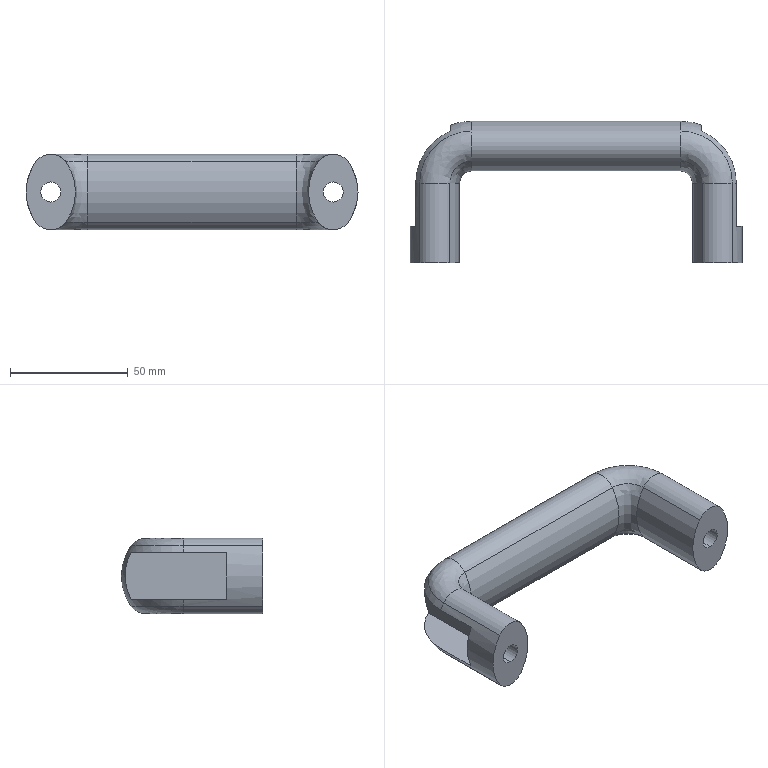Part | SolidWorks | features BaseBody 1 | 1 solid | 43 faces | box 141 x 60 x 32 mm | volume 81760 mm3 | cylinder 23 | plane 12 | spline 8 | commonest cylinder face diameters 16 x9 44.044 x6 8.5 x4 13.5 x4
STEP:
#1=CARTESIAN_POINT('',(-44.25,43.137,-12.848));
#2=VERTEX_POINT('',#1);
#3=CARTESIAN_POINT('',(-44.25,49.5,-16.));
#4=VERTEX_POINT('',#3);
#5=CARTESIAN_POINT('',(-44.25,49.5,-8.));
#6=DIRECTION('',(1.,0.,0.));
#7=DIRECTION('',(0.,0.,-1.));
#8=AXIS2_PLACEMENT_3D('',#5,#6,#7);
#9=CIRCLE('',#8,8.);
#10=EDGE_CURVE('',#2,#4,#9,.T.);
#11=ORIENTED_EDGE('',*,*,#10,.T.);
#12=CARTESIAN_POINT('',(44.25,49.5,-16.));
#13=VERTEX_POINT('',#12);
#14=CARTESIAN_POINT('',(44.25,49.5,-16.));
#15=DIRECTION('',(1.,0.,0.));
#16=VECTOR('',#15,1000.);
#17=LINE('',#14,#16);
#18=EDGE_CURVE('',#4,#13,#17,.T.);
#19=ORIENTED_EDGE('',*,*,#18,.T.);
#20=CARTESIAN_POINT('',(44.25,43.137,-12.848));
#21=VERTEX_POINT('',#20);
#22=CARTESIAN_POINT('',(44.25,49.5,-8.));
#23=DIRECTION('',(-1.,0.,0.));
#24=DIRECTION('',(0.,0.,-1.));
#25=AXIS2_PLACEMENT_3D('',#22,#23,#24);
#26=CIRCLE('',#25,8.);
#27=EDGE_CURVE('',#13,#21,#26,.T.);
#28=ORIENTED_EDGE('',*,*,#27,.T.);
#29=CARTESIAN_POINT('',(44.25,43.137,-12.848));
#30=DIRECTION('',(1.,0.,0.));
#31=VECTOR('',#30,1000.);
#32=LINE('',#29,#31);
#33=EDGE_CURVE('',#2,#21,#32,.T.);
#34=ORIENTED_EDGE('',*,*,#33,.F.);
#35=EDGE_LOOP('',(#11,#19,#28,#34));
#36=FACE_OUTER_BOUND('',#35,.T.);
#37=CARTESIAN_POINT('',(44.25,49.5,-8.));
#38=DIRECTION('',(1.,0.,0.));
#39=DIRECTION('',(0.,0.,-1.));
#40=AXIS2_PLACEMENT_3D('',#37,#38,#39);
#41=CYLINDRICAL_SURFACE('',#40,8.);
#42=ADVANCED_FACE('',(#36),#41,.T.);
#43=CARTESIAN_POINT('',(60.,33.75,-16.));
#44=VERTEX_POINT('',#43);
#45=CARTESIAN_POINT('',(53.637,33.75,-12.848));
#46=VERTEX_POINT('',#45);
#47=CARTESIAN_POINT('',(60.,33.75,-8.));
#48=DIRECTION('',(0.,1.,0.));
#49=DIRECTION('',(1.,0.,0.));
#50=AXIS2_PLACEMENT_3D('',#47,#48,#49);
#51=CIRCLE('',#50,8.);
#52=EDGE_CURVE('',#44,#46,#51,.T.);
#53=ORIENTED_EDGE('',*,*,#52,.F.);
#54=CARTESIAN_POINT('',(60.,0.,-16.));
#55=VERTEX_POINT('',#54);
#56=CARTESIAN_POINT('',(60.,0.,-16.));
#57=DIRECTION('',(0.,-1.,0.));
#58=VECTOR('',#57,1000.);
#59=LINE('',#56,#58);
#60=EDGE_CURVE('',#44,#55,#59,.T.);
#61=ORIENTED_EDGE('',*,*,#60,.T.);
#62=CARTESIAN_POINT('',(53.637,0.,-12.848));
#63=VERTEX_POINT('',#62);
#64=CARTESIAN_POINT('',(60.,0.,-8.));
#65=DIRECTION('',(0.,1.,0.));
#66=DIRECTION('',(0.,0.,-1.));
#67=AXIS2_PLACEMENT_3D('',#64,#65,#66);
#68=CIRCLE('',#67,8.);
#69=EDGE_CURVE('',#55,#63,#68,.T.);
#70=ORIENTED_EDGE('',*,*,#69,.T.);
#71=CARTESIAN_POINT('',(53.637,0.,-12.848));
#72=DIRECTION('',(0.,-1.,0.));
#73=VECTOR('',#72,1000.);
#74=LINE('',#71,#73);
#75=EDGE_CURVE('',#46,#63,#74,.T.);
#76=ORIENTED_EDGE('',*,*,#75,.F.);
#77=EDGE_LOOP('',(#53,#61,#70,#76));
#78=FACE_OUTER_BOUND('',#77,.T.);
#79=CARTESIAN_POINT('',(60.,0.,-8.));
#80=DIRECTION('',(0.,-1.,0.));
#81=DIRECTION('',(0.,0.,-1.));
#82=AXIS2_PLACEMENT_3D('',#79,#80,#81);
#83=CYLINDRICAL_SURFACE('',#82,8.);
#84=ADVANCED_FACE('',(#78),#83,.T.);
#85=CARTESIAN_POINT('',(-60.,33.75,-16.));
#86=VERTEX_POINT('',#85);
#87=CARTESIAN_POINT('',(-66.363,33.75,-12.848));
#88=VERTEX_POINT('',#87);
#89=CARTESIAN_POINT('',(-60.,33.75,-8.));
#90=DIRECTION('',(0.,1.,0.));
#91=DIRECTION('',(-1.,0.,0.));
#92=AXIS2_PLACEMENT_3D('',#89,#90,#91);
#93=CIRCLE('',#92,8.);
#94=EDGE_CURVE('',#86,#88,#93,.T.);
#95=ORIENTED_EDGE('',*,*,#94,.F.);
#96=CARTESIAN_POINT('',(-60.,0.,-16.));
#97=VERTEX_POINT('',#96);
#98=CARTESIAN_POINT('',(-60.,0.,-16.));
#99=DIRECTION('',(0.,-1.,0.));
#100=VECTOR('',#99,1000.);
#101=LINE('',#98,#100);
#102=EDGE_CURVE('',#86,#97,#101,.T.);
#103=ORIENTED_EDGE('',*,*,#102,.T.);
#104=CARTESIAN_POINT('',(-66.363,0.,-12.848));
#105=VERTEX_POINT('',#104);
#106=CARTESIAN_POINT('',(-60.,0.,-8.));
#107=DIRECTION('',(0.,1.,0.));
#108=DIRECTION('',(0.,0.,-1.));
#109=AXIS2_PLACEMENT_3D('',#106,#107,#108);
#110=CIRCLE('',#109,8.);
#111=EDGE_CURVE('',#97,#105,#110,.T.);
#112=ORIENTED_EDGE('',*,*,#111,.T.);
#113=CARTESIAN_POINT('',(-66.363,0.,-12.848));
#114=DIRECTION('',(0.,1.,0.));
#115=VECTOR('',#114,1000.);
#116=LINE('',#113,#115);
#117=EDGE_CURVE('',#105,#88,#116,.T.);
#118=ORIENTED_EDGE('',*,*,#117,.T.);
#119=EDGE_LOOP('',(#95,#103,#112,#118));
#120=FACE_OUTER_BOUND('',#119,.T.);
#121=CARTESIAN_POINT('',(-60.,0.,-8.));
#122=DIRECTION('',(0.,-1.,0.));
#123=DIRECTION('',(0.,0.,-1.));
#124=AXIS2_PLACEMENT_3D('',#121,#122,#123);
#125=CYLINDRICAL_SURFACE('',#124,8.);
#126=ADVANCED_FACE('',(#120),#125,.T.);
#127=CARTESIAN_POINT('',(60.,7.,4.25));
#128=VERTEX_POINT('',#127);
#129=CARTESIAN_POINT('',(60.,7.,-4.25));
#130=VERTEX_POINT('',#129);
#131=CARTESIAN_POINT('',(60.,7.,0.));
#132=DIRECTION('',(0.,-1.,0.));
#133=DIRECTION('',(0.,0.,-1.));
#134=AXIS2_PLACEMENT_3D('',#131,#132,#133);
#135=CIRCLE('',#134,4.25);
#136=EDGE_CURVE('',#128,#130,#135,.T.);
#137=ORIENTED_EDGE('',*,*,#136,.F.);
#138=CARTESIAN_POINT('',(60.,0.,4.25));
#139=VERTEX_POINT('',#138);
#140=CARTESIAN_POINT('',(60.,3.5,4.25));
#141=DIRECTION('',(0.,-1.,0.));
#142=VECTOR('',#141,1000.);
#143=LINE('',#140,#142);
#144=EDGE_CURVE('',#128,#139,#143,.T.);
#145=ORIENTED_EDGE('',*,*,#144,.T.);
#146=CARTESIAN_POINT('',(60.,0.,-4.25));
#147=VERTEX_POINT('',#146);
#148=CARTESIAN_POINT('',(60.,0.,0.));
#149=DIRECTION('',(0.,-1.,0.));
#150=DIRECTION('',(0.,0.,-1.));
#151=AXIS2_PLACEMENT_3D('',#148,#149,#150);
#152=CIRCLE('',#151,4.25);
#153=EDGE_CURVE('',#139,#147,#152,.T.);
#154=ORIENTED_EDGE('',*,*,#153,.T.);
#155=CARTESIAN_POINT('',(60.,3.5,-4.25));
#156=DIRECTION('',(0.,-1.,0.));
#157=VECTOR('',#156,1000.);
#158=LINE('',#155,#157);
#159=EDGE_CURVE('',#130,#147,#158,.T.);
#160=ORIENTED_EDGE('',*,*,#159,.F.);
#161=EDGE_LOOP('',(#137,#145,#154,#160));
#162=FACE_OUTER_BOUND('',#161,.T.);
#163=CARTESIAN_POINT('',(60.,3.5,0.));
#164=DIRECTION('',(0.,-1.,0.));
#165=DIRECTION('',(0.,0.,-1.));
#166=AXIS2_PLACEMENT_3D('',#163,#164,#165);
#167=CYLINDRICAL_SURFACE('',#166,4.25);
#168=ADVANCED_FACE('',(#162),#167,.F.);
#169=CARTESIAN_POINT('',(-60.,7.,4.25));
#170=VERTEX_POINT('',#169);
#171=CARTESIAN_POINT('',(-60.,7.,-4.25));
#172=VERTEX_POINT('',#171);
#173=CARTESIAN_POINT('',(-60.,7.,0.));
#174=DIRECTION('',(0.,-1.,0.));
#175=DIRECTION('',(0.,0.,-1.));
#176=AXIS2_PLACEMENT_3D('',#173,#174,#175);
#177=CIRCLE('',#176,4.25);
#178=EDGE_CURVE('',#170,#172,#177,.T.);
#179=ORIENTED_EDGE('',*,*,#178,.F.);
#180=CARTESIAN_POINT('',(-60.,0.,4.25));
#181=VERTEX_POINT('',#180);
#182=CARTESIAN_POINT('',(-60.,3.5,4.25));
#183=DIRECTION('',(0.,-1.,0.));
#184=VECTOR('',#183,1000.);
#185=LINE('',#182,#184);
#186=EDGE_CURVE('',#170,#181,#185,.T.);
#187=ORIENTED_EDGE('',*,*,#186,.T.);
#188=CARTESIAN_POINT('',(-60.,0.,-4.25));
#189=VERTEX_POINT('',#188);
#190=CARTESIAN_POINT('',(-60.,0.,0.));
#191=DIRECTION('',(0.,-1.,0.));
#192=DIRECTION('',(0.,0.,-1.));
#193=AXIS2_PLACEMENT_3D('',#190,#191,#192);
#194=CIRCLE('',#193,4.25);
#195=EDGE_CURVE('',#181,#189,#194,.T.);
#196=ORIENTED_EDGE('',*,*,#195,.T.);
#197=CARTESIAN_POINT('',(-60.,3.5,-4.25));
#198=DIRECTION('',(0.,-1.,0.));
#199=VECTOR('',#198,1000.);
#200=LINE('',#197,#199);
#201=EDGE_CURVE('',#172,#189,#200,.T.);
#202=ORIENTED_EDGE('',*,*,#201,.F.);
#203=EDGE_LOOP('',(#179,#187,#196,#202));
#204=FACE_OUTER_BOUND('',#203,.T.);
#205=CARTESIAN_POINT('',(-60.,3.5,0.));
#206=DIRECTION('',(0.,-1.,0.));
#207=DIRECTION('',(0.,0.,-1.));
#208=AXIS2_PLACEMENT_3D('',#205,#206,#207);
#209=CYLINDRICAL_SURFACE('',#208,4.25);
#210=ADVANCED_FACE('',(#204),#209,.F.);
#211=CARTESIAN_POINT('',(60.,15.5,-6.75));
#212=VERTEX_POINT('',#211);
#213=CARTESIAN_POINT('',(60.,15.5,6.75));
#214=VERTEX_POINT('',#213);
#215=CARTESIAN_POINT('',(60.,15.5,0.));
#216=DIRECTION('',(0.,1.,0.));
#217=DIRECTION('',(0.,0.,-1.));
#218=AXIS2_PLACEMENT_3D('',#215,#216,#217);
#219=CIRCLE('',#218,6.75);
#220=EDGE_CURVE('',#212,#214,#219,.T.);
#221=ORIENTED_EDGE('',*,*,#220,.T.);
#222=CARTESIAN_POINT('',(60.,7.,6.75));
#223=VERTEX_POINT('',#222);
#224=CARTESIAN_POINT('',(60.,11.25,6.75));
#225=DIRECTION('',(0.,-1.,0.));
#226=VECTOR('',#225,1000.);
#227=LINE('',#224,#226);
#228=EDGE_CURVE('',#214,#223,#227,.T.);
#229=ORIENTED_EDGE('',*,*,#228,.T.);
#230=CARTESIAN_POINT('',(60.,7.,-6.75));
#231=VERTEX_POINT('',#230);
#232=CARTESIAN_POINT('',(60.,7.,0.));
#233=DIRECTION('',(0.,-1.,0.));
#234=DIRECTION('',(0.,0.,-1.));
#235=AXIS2_PLACEMENT_3D('',#232,#233,#234);
#236=CIRCLE('',#235,6.75);
#237=EDGE_CURVE('',#223,#231,#236,.T.);
#238=ORIENTED_EDGE('',*,*,#237,.T.);
#239=CARTESIAN_POINT('',(60.,11.25,-6.75));
#240=DIRECTION('',(0.,-1.,0.));
#241=VECTOR('',#240,1000.);
#242=LINE('',#239,#241);
#243=EDGE_CURVE('',#212,#231,#242,.T.);
#244=ORIENTED_EDGE('',*,*,#243,.F.);
#245=EDGE_LOOP('',(#221,#229,#238,#244));
#246=FACE_OUTER_BOUND('',#245,.T.);
#247=CARTESIAN_POINT('',(60.,11.25,0.));
#248=DIRECTION('',(0.,-1.,0.));
#249=DIRECTION('',(0.,0.,-1.));
#250=AXIS2_PLACEMENT_3D('',#247,#248,#249);
#251=CYLINDRICAL_SURFACE('',#250,6.75);
#252=ADVANCED_FACE('',(#246),#251,.F.);
#253=CARTESIAN_POINT('',(-60.,15.5,-6.75));
#254=VERTEX_POINT('',#253);
#255=CARTESIAN_POINT('',(-60.,15.5,6.75));
#256=VERTEX_POINT('',#255);
#257=CARTESIAN_POINT('',(-60.,15.5,0.));
#258=DIRECTION('',(0.,1.,0.));
#259=DIRECTION('',(0.,0.,-1.));
#260=AXIS2_PLACEMENT_3D('',#257,#258,#259);
#261=CIRCLE('',#260,6.75);
#262=EDGE_CURVE('',#254,#256,#261,.T.);
#263=ORIENTED_EDGE('',*,*,#262,.T.);
#264=CARTESIAN_POINT('',(-60.,7.,6.75));
#265=VERTEX_POINT('',#264);
#266=CARTESIAN_POINT('',(-60.,11.25,6.75));
#267=DIRECTION('',(0.,-1.,0.));
#268=VECTOR('',#267,1000.);
#269=LINE('',#266,#268);
#270=EDGE_CURVE('',#256,#265,#269,.T.);
#271=ORIENTED_EDGE('',*,*,#270,.T.);
#272=CARTESIAN_POINT('',(-60.,7.,-6.75));
#273=VERTEX_POINT('',#272);
#274=CARTESIAN_POINT('',(-60.,7.,0.));
#275=DIRECTION('',(0.,-1.,0.));
#276=DIRECTION('',(0.,0.,-1.));
#277=AXIS2_PLACEMENT_3D('',#274,#275,#276);
#278=CIRCLE('',#277,6.75);
#279=EDGE_CURVE('',#265,#273,#278,.T.);
#280=ORIENTED_EDGE('',*,*,#279,.T.);
#281=CARTESIAN_POINT('',(-60.,11.25,-6.75));
#282=DIRECTION('',(0.,-1.,0.));
#283=VECTOR('',#282,1000.);
#284=LINE('',#281,#283);
#285=EDGE_CURVE('',#254,#273,#284,.T.);
#286=ORIENTED_EDGE('',*,*,#285,.F.);
#287=EDGE_LOOP('',(#263,#271,#280,#286));
#288=FACE_OUTER_BOUND('',#287,.T.);
#289=CARTESIAN_POINT('',(-60.,11.25,0.));
#290=DIRECTION('',(0.,-1.,0.));
#291=DIRECTION('',(0.,0.,-1.));
#292=AXIS2_PLACEMENT_3D('',#289,#290,#291);
#293=CYLINDRICAL_SURFACE('',#292,6.75);
#294=ADVANCED_FACE('',(#288),#293,.F.);
#295=CARTESIAN_POINT('',(44.25,43.137,12.848));
#296=VERTEX_POINT('',#295);
#297=CARTESIAN_POINT('',(44.25,61.022,0.));
#298=DIRECTION('',(-1.,0.,0.));
#299=DIRECTION('',(0.,0.,-1.));
#300=AXIS2_PLACEMENT_3D('',#297,#298,#299);
#301=CIRCLE('',#300,22.022);
#302=EDGE_CURVE('',#21,#296,#301,.T.);
#303=ORIENTED_EDGE('',*,*,#302,.T.);
#304=CARTESIAN_POINT('',(-44.25,43.137,12.848));
#305=VERTEX_POINT('',#304);
#306=CARTESIAN_POINT('',(44.25,43.137,12.848));
#307=DIRECTION('',(-1.,0.,0.));
#308=VECTOR('',#307,1000.);
#309=LINE('',#306,#308);
#310=EDGE_CURVE('',#296,#305,#309,.T.);
#311=ORIENTED_EDGE('',*,*,#310,.T.);
#312=CARTESIAN_POINT('',(-44.25,61.022,0.));
#313=DIRECTION('',(1.,0.,0.));
#314=DIRECTION('',(0.,0.,-1.));
#315=AXIS2_PLACEMENT_3D('',#312,#313,#314);
#316=CIRCLE('',#315,22.022);
#317=EDGE_CURVE('',#305,#2,#316,.T.);
#318=ORIENTED_EDGE('',*,*,#317,.T.);
#319=ORIENTED_EDGE('',*,*,#33,.T.);
#320=EDGE_LOOP('',(#303,#311,#318,#319));
#321=FACE_OUTER_BOUND('',#320,.T.);
#322=CARTESIAN_POINT('',(44.25,61.022,0.));
#323=DIRECTION('',(1.,0.,0.));
#324=DIRECTION('',(0.,0.,-1.));
#325=AXIS2_PLACEMENT_3D('',#322,#323,#324);
#326=CYLINDRICAL_SURFACE('',#325,22.022);
#327=ADVANCED_FACE('',(#321),#326,.T.);
#328=CARTESIAN_POINT('',(44.25,55.863,12.848));
#329=VERTEX_POINT('',#328);
#330=CARTESIAN_POINT('',(44.25,49.5,8.));
#331=DIRECTION('',(-1.,0.,0.));
#332=DIRECTION('',(0.,0.,-1.));
#333=AXIS2_PLACEMENT_3D('',#330,#331,#332);
#334=CIRCLE('',#333,8.);
#335=EDGE_CURVE('',#296,#329,#334,.T.);
#336=ORIENTED_EDGE('',*,*,#335,.T.);
#337=CARTESIAN_POINT('',(-44.25,55.863,12.848));
#338=VERTEX_POINT('',#337);
#339=CARTESIAN_POINT('',(44.25,55.863,12.848));
#340=DIRECTION('',(-1.,0.,0.));
#341=VECTOR('',#340,1000.);
#342=LINE('',#339,#341);
#343=EDGE_CURVE('',#329,#338,#342,.T.);
#344=ORIENTED_EDGE('',*,*,#343,.T.);
#345=CARTESIAN_POINT('',(-44.25,49.5,8.));
#346=DIRECTION('',(1.,0.,0.));
#347=DIRECTION('',(0.,0.,-1.));
#348=AXIS2_PLACEMENT_3D('',#345,#346,#347);
#349=CIRCLE('',#348,8.);
#350=EDGE_CURVE('',#338,#305,#349,.T.);
#351=ORIENTED_EDGE('',*,*,#350,.T.);
#352=ORIENTED_EDGE('',*,*,#310,.F.);
#353=EDGE_LOOP('',(#336,#344,#351,#352));
#354=FACE_OUTER_BOUND('',#353,.T.);
#355=CARTESIAN_POINT('',(44.25,49.5,8.));
#356=DIRECTION('',(1.,0.,0.));
#357=DIRECTION('',(0.,0.,-1.));
#358=AXIS2_PLACEMENT_3D('',#355,#356,#357);
#359=CYLINDRICAL_SURFACE('',#358,8.);
#360=ADVANCED_FACE('',(#354),#359,.T.);
#361=CARTESIAN_POINT('',(53.637,33.75,12.848));
#362=VERTEX_POINT('',#361);
#363=CARTESIAN_POINT('',(44.25,33.75,12.848));
#364=DIRECTION('',(0.,0.,1.));
#365=DIRECTION('',(1.,0.,0.));
#366=AXIS2_PLACEMENT_3D('',#363,#364,#365);
#367=CIRCLE('',#366,9.387);
#368=EDGE_CURVE('',#362,#296,#367,.T.);
#369=ORIENTED_EDGE('',*,*,#368,.T.);
#370=ORIENTED_EDGE('',*,*,#302,.F.);
#371=CARTESIAN_POINT('',(44.25,33.75,-12.848));
#372=DIRECTION('',(0.,0.,-1.));
#373=DIRECTION('',(1.,0.,0.));
#374=AXIS2_PLACEMENT_3D('',#371,#372,#373);
#375=CIRCLE('',#374,9.387);
#376=EDGE_CURVE('',#21,#46,#375,.T.);
#377=ORIENTED_EDGE('',*,*,#376,.T.);
#378=CARTESIAN_POINT('',(71.522,33.75,0.));
#379=DIRECTION('',(0.,1.,0.));
#380=DIRECTION('',(1.,0.,0.));
#381=AXIS2_PLACEMENT_3D('',#378,#379,#380);
#382=CIRCLE('',#381,22.022);
#383=EDGE_CURVE('',#46,#362,#382,.T.);
#384=ORIENTED_EDGE('',*,*,#383,.T.);
#385=EDGE_LOOP('',(#369,#370,#377,#384));
#386=FACE_OUTER_BOUND('',#385,.T.);
#387=CARTESIAN_POINT('',(53.637,33.75,-12.848));
#388=CARTESIAN_POINT('',(53.637,39.249,-12.848));
#389=CARTESIAN_POINT('',(49.749,43.137,-12.848));
#390=CARTESIAN_POINT('',(44.25,43.137,-12.848));
#391=CARTESIAN_POINT('',(47.924,33.75,-4.896));
#392=CARTESIAN_POINT('',(47.924,35.902,-4.896));
#393=CARTESIAN_POINT('',(46.402,37.424,-4.896));
#394=CARTESIAN_POINT('',(44.25,37.424,-4.896));
#395=CARTESIAN_POINT('',(47.924,33.75,4.896));
#396=CARTESIAN_POINT('',(47.924,35.902,4.896));
#397=CARTESIAN_POINT('',(46.402,37.424,4.896));
#398=CARTESIAN_POINT('',(44.25,37.424,4.896));
#399=CARTESIAN_POINT('',(53.637,33.75,12.848));
#400=CARTESIAN_POINT('',(53.637,39.249,12.848));
#401=CARTESIAN_POINT('',(49.749,43.137,12.848));
#402=CARTESIAN_POINT('',(44.25,43.137,12.848));
#403=(BOUNDED_SURFACE()B_SPLINE_SURFACE(3,3,((#387,#388,#389,#390),(#391,#392,#393,#394),(#395,#396,#397,#398),(#399,#400,#401,#402)),.UNSPECIFIED.,.F.,.F.,.T.)B_SPLINE_SURFACE_WITH_KNOTS((4,4),(4,4),(0.,1.),(0.,1.),.UNSPECIFIED.)GEOMETRIC_REPRESENTATION_ITEM()RATIONAL_B_SPLINE_SURFACE(((1.,0.8047,0.8047,1.),(0.8748,0.704,0.704,0.8748),(0.8748,0.704,0.704,0.8748),(1.,0.8047,0.8047,1.)))REPRESENTATION_ITEM('')SURFACE());
#404=ADVANCED_FACE('',(#386),#403,.T.);
#405=ORIENTED_EDGE('',*,*,#18,.F.);
#406=CARTESIAN_POINT('',(-44.25,55.863,-12.848));
#407=VERTEX_POINT('',#406);
#408=CARTESIAN_POINT('',(-44.25,49.5,-8.));
#409=DIRECTION('',(1.,0.,0.));
#410=DIRECTION('',(0.,0.,-1.));
#411=AXIS2_PLACEMENT_3D('',#408,#409,#410);
#412=CIRCLE('',#411,8.);
#413=EDGE_CURVE('',#4,#407,#412,.T.);
#414=ORIENTED_EDGE('',*,*,#413,.T.);
#415=CARTESIAN_POINT('',(44.25,55.863,-12.848));
#416=VERTEX_POINT('',#415);
#417=CARTESIAN_POINT('',(44.25,55.863,-12.848));
#418=DIRECTION('',(1.,0.,0.));
#419=VECTOR('',#418,1000.);
#420=LINE('',#417,#419);
#421=EDGE_CURVE('',#407,#416,#420,.T.);
#422=ORIENTED_EDGE('',*,*,#421,.T.);
#423=CARTESIAN_POINT('',(44.25,49.5,-8.));
#424=DIRECTION('',(-1.,0.,0.));
#425=DIRECTION('',(0.,0.,-1.));
#426=AXIS2_PLACEMENT_3D('',#423,#424,#425);
#427=CIRCLE('',#426,8.);
#428=EDGE_CURVE('',#416,#13,#427,.T.);
#429=ORIENTED_EDGE('',*,*,#428,.T.);
#430=EDGE_LOOP('',(#405,#414,#422,#429));
#431=FACE_OUTER_BOUND('',#430,.T.);
#432=CARTESIAN_POINT('',(44.25,49.5,-8.));
#433=DIRECTION('',(1.,0.,0.));
#434=DIRECTION('',(0.,0.,-1.));
#435=AXIS2_PLACEMENT_3D('',#432,#433,#434);
#436=CYLINDRICAL_SURFACE('',#435,8.);
#437=ADVANCED_FACE('',(#431),#436,.T.);
#438=CARTESIAN_POINT('',(-53.637,33.75,-12.848));
#439=VERTEX_POINT('',#438);
#440=CARTESIAN_POINT('',(-44.25,33.75,-12.848));
#441=DIRECTION('',(0.,0.,-1.));
#442=DIRECTION('',(-1.,0.,0.));
#443=AXIS2_PLACEMENT_3D('',#440,#441,#442);
#444=CIRCLE('',#443,9.387);
#445=EDGE_CURVE('',#439,#2,#444,.T.);
#446=ORIENTED_EDGE('',*,*,#445,.T.);
#447=ORIENTED_EDGE('',*,*,#317,.F.);
#448=CARTESIAN_POINT('',(-53.637,33.75,12.848));
#449=VERTEX_POINT('',#448);
#450=CARTESIAN_POINT('',(-44.25,33.75,12.848));
#451=DIRECTION('',(0.,0.,1.));
#452=DIRECTION('',(-1.,0.,0.));
#453=AXIS2_PLACEMENT_3D('',#450,#451,#452);
#454=CIRCLE('',#453,9.387);
#455=EDGE_CURVE('',#305,#449,#454,.T.);
#456=ORIENTED_EDGE('',*,*,#455,.T.);
#457=CARTESIAN_POINT('',(-71.522,33.75,0.));
#458=DIRECTION('',(0.,1.,0.));
#459=DIRECTION('',(-1.,0.,0.));
#460=AXIS2_PLACEMENT_3D('',#457,#458,#459);
#461=CIRCLE('',#460,22.022);
#462=EDGE_CURVE('',#449,#439,#461,.T.);
#463=ORIENTED_EDGE('',*,*,#462,.T.);
#464=EDGE_LOOP('',(#446,#447,#456,#463));
#465=FACE_OUTER_BOUND('',#464,.T.);
#466=CARTESIAN_POINT('',(-53.637,33.75,12.848));
#467=CARTESIAN_POINT('',(-53.637,39.249,12.848));
#468=CARTESIAN_POINT('',(-49.749,43.137,12.848));
#469=CARTESIAN_POINT('',(-44.25,43.137,12.848));
#470=CARTESIAN_POINT('',(-47.924,33.75,4.896));
#471=CARTESIAN_POINT('',(-47.924,35.902,4.896));
#472=CARTESIAN_POINT('',(-46.402,37.424,4.896));
#473=CARTESIAN_POINT('',(-44.25,37.424,4.896));
#474=CARTESIAN_POINT('',(-47.924,33.75,-4.896));
#475=CARTESIAN_POINT('',(-47.924,35.902,-4.896));
#476=CARTESIAN_POINT('',(-46.402,37.424,-4.896));
#477=CARTESIAN_POINT('',(-44.25,37.424,-4.896));
#478=CARTESIAN_POINT('',(-53.637,33.75,-12.848));
#479=CARTESIAN_POINT('',(-53.637,39.249,-12.848));
#480=CARTESIAN_POINT('',(-49.749,43.137,-12.848));
#481=CARTESIAN_POINT('',(-44.25,43.137,-12.848));
#482=(BOUNDED_SURFACE()B_SPLINE_SURFACE(3,3,((#466,#467,#468,#469),(#470,#471,#472,#473),(#474,#475,#476,#477),(#478,#479,#480,#481)),.UNSPECIFIED.,.F.,.F.,.T.)B_SPLINE_SURFACE_WITH_KNOTS((4,4),(4,4),(0.,1.),(0.,1.),.UNSPECIFIED.)GEOMETRIC_REPRESENTATION_ITEM()RATIONAL_B_SPLINE_SURFACE(((1.,0.8047,0.8047,1.),(0.8748,0.704,0.704,0.8748),(0.8748,0.704,0.704,0.8748),(1.,0.8047,0.8047,1.)))REPRESENTATION_ITEM('')SURFACE());
#483=ADVANCED_FACE('',(#465),#482,.T.);
#484=CARTESIAN_POINT('',(44.25,37.978,0.));
#485=DIRECTION('',(-1.,0.,0.));
#486=DIRECTION('',(0.,0.,-1.));
#487=AXIS2_PLACEMENT_3D('',#484,#485,#486);
#488=CIRCLE('',#487,22.022);
#489=EDGE_CURVE('',#329,#416,#488,.T.);
#490=ORIENTED_EDGE('',*,*,#489,.T.);
#491=ORIENTED_EDGE('',*,*,#421,.F.);
#492=CARTESIAN_POINT('',(-44.25,37.978,0.));
#493=DIRECTION('',(1.,0.,0.));
#494=DIRECTION('',(0.,0.,-1.));
#495=AXIS2_PLACEMENT_3D('',#492,#493,#494);
#496=CIRCLE('',#495,22.022);
#497=EDGE_CURVE('',#407,#338,#496,.T.);
#498=ORIENTED_EDGE('',*,*,#497,.T.);
#499=ORIENTED_EDGE('',*,*,#343,.F.);
#500=EDGE_LOOP('',(#490,#491,#498,#499));
#501=FACE_OUTER_BOUND('',#500,.T.);
#502=CARTESIAN_POINT('',(44.25,37.978,0.));
#503=DIRECTION('',(1.,0.,0.));
#504=DIRECTION('',(0.,0.,-1.));
#505=AXIS2_PLACEMENT_3D('',#502,#503,#504);
#506=CYLINDRICAL_SURFACE('',#505,22.022);
#507=ADVANCED_FACE('',(#501),#506,.T.);
#508=CARTESIAN_POINT('',(66.363,33.75,12.848));
#509=VERTEX_POINT('',#508);
#510=CARTESIAN_POINT('',(60.,33.75,8.));
#511=DIRECTION('',(0.,1.,0.));
#512=DIRECTION('',(1.,0.,0.));
#513=AXIS2_PLACEMENT_3D('',#510,#511,#512);
#514=CIRCLE('',#513,8.);
#515=EDGE_CURVE('',#362,#509,#514,.T.);
#516=ORIENTED_EDGE('',*,*,#515,.T.);
#517=CARTESIAN_POINT('',(44.25,33.75,12.848));
#518=DIRECTION('',(0.,0.,1.));
#519=DIRECTION('',(1.,0.,0.));
#520=AXIS2_PLACEMENT_3D('',#517,#518,#519);
#521=CIRCLE('',#520,22.113);
#522=EDGE_CURVE('',#509,#329,#521,.T.);
#523=ORIENTED_EDGE('',*,*,#522,.T.);
#524=ORIENTED_EDGE('',*,*,#335,.F.);
#525=ORIENTED_EDGE('',*,*,#368,.F.);
#526=EDGE_LOOP('',(#516,#523,#524,#525));
#527=FACE_OUTER_BOUND('',#526,.T.);
#528=CARTESIAN_POINT('',(53.637,33.75,12.848));
#529=CARTESIAN_POINT('',(53.637,39.249,12.848));
#530=CARTESIAN_POINT('',(49.749,43.137,12.848));
#531=CARTESIAN_POINT('',(44.25,43.137,12.848));
#532=CARTESIAN_POINT('',(57.123,33.75,17.425));
#533=CARTESIAN_POINT('',(57.123,41.291,17.425));
#534=CARTESIAN_POINT('',(51.791,46.623,17.425));
#535=CARTESIAN_POINT('',(44.25,46.623,17.425));
#536=CARTESIAN_POINT('',(62.877,33.75,17.425));
#537=CARTESIAN_POINT('',(62.877,44.661,17.425));
#538=CARTESIAN_POINT('',(55.161,52.377,17.425));
#539=CARTESIAN_POINT('',(44.25,52.377,17.425));
#540=CARTESIAN_POINT('',(66.363,33.75,12.848));
#541=CARTESIAN_POINT('',(66.363,46.704,12.848));
#542=CARTESIAN_POINT('',(57.204,55.863,12.848));
#543=CARTESIAN_POINT('',(44.25,55.863,12.848));
#544=(BOUNDED_SURFACE()B_SPLINE_SURFACE(3,3,((#528,#529,#530,#531),(#532,#533,#534,#535),(#536,#537,#538,#539),(#540,#541,#542,#543)),.UNSPECIFIED.,.F.,.F.,.F.)B_SPLINE_SURFACE_WITH_KNOTS((4,4),(4,4),(0.,1.),(0.,1.),.UNSPECIFIED.)GEOMETRIC_REPRESENTATION_ITEM()RATIONAL_B_SPLINE_SURFACE(((1.,0.8047,0.8047,1.),(0.7374,0.5934,0.5934,0.7374),(0.7374,0.5934,0.5934,0.7374),(1.,0.8047,0.8047,1.)))REPRESENTATION_ITEM('')SURFACE());
#545=ADVANCED_FACE('',(#527),#544,.T.);
#546=CARTESIAN_POINT('',(-66.363,33.75,12.848));
#547=VERTEX_POINT('',#546);
#548=CARTESIAN_POINT('',(-60.,33.75,8.));
#549=DIRECTION('',(0.,1.,0.));
#550=DIRECTION('',(-1.,0.,0.));
#551=AXIS2_PLACEMENT_3D('',#548,#549,#550);
#552=CIRCLE('',#551,8.);
#553=EDGE_CURVE('',#547,#449,#552,.T.);
#554=ORIENTED_EDGE('',*,*,#553,.T.);
#555=ORIENTED_EDGE('',*,*,#455,.F.);
#556=ORIENTED_EDGE('',*,*,#350,.F.);
#557=CARTESIAN_POINT('',(-44.25,33.75,12.848));
#558=DIRECTION('',(0.,0.,1.));
#559=DIRECTION('',(-1.,0.,0.));
#560=AXIS2_PLACEMENT_3D('',#557,#558,#559);
#561=CIRCLE('',#560,22.113);
#562=EDGE_CURVE('',#338,#547,#561,.T.);
#563=ORIENTED_EDGE('',*,*,#562,.T.);
#564=EDGE_LOOP('',(#554,#555,#556,#563));
#565=FACE_OUTER_BOUND('',#564,.T.);
#566=CARTESIAN_POINT('',(-66.363,33.75,12.848));
#567=CARTESIAN_POINT('',(-66.363,46.704,12.848));
#568=CARTESIAN_POINT('',(-57.204,55.863,12.848));
#569=CARTESIAN_POINT('',(-44.25,55.863,12.848));
#570=CARTESIAN_POINT('',(-62.877,33.75,17.425));
#571=CARTESIAN_POINT('',(-62.877,44.661,17.425));
#572=CARTESIAN_POINT('',(-55.161,52.377,17.425));
#573=CARTESIAN_POINT('',(-44.25,52.377,17.425));
#574=CARTESIAN_POINT('',(-57.123,33.75,17.425));
#575=CARTESIAN_POINT('',(-57.123,41.291,17.425));
#576=CARTESIAN_POINT('',(-51.791,46.623,17.425));
#577=CARTESIAN_POINT('',(-44.25,46.623,17.425));
#578=CARTESIAN_POINT('',(-53.637,33.75,12.848));
#579=CARTESIAN_POINT('',(-53.637,39.249,12.848));
#580=CARTESIAN_POINT('',(-49.749,43.137,12.848));
#581=CARTESIAN_POINT('',(-44.25,43.137,12.848));
#582=(BOUNDED_SURFACE()B_SPLINE_SURFACE(3,3,((#566,#567,#568,#569),(#570,#571,#572,#573),(#574,#575,#576,#577),(#578,#579,#580,#581)),.UNSPECIFIED.,.F.,.F.,.T.)B_SPLINE_SURFACE_WITH_KNOTS((4,4),(4,4),(0.,1.),(0.,1.),.UNSPECIFIED.)GEOMETRIC_REPRESENTATION_ITEM()RATIONAL_B_SPLINE_SURFACE(((1.,0.8047,0.8047,1.),(0.7374,0.5934,0.5934,0.7374),(0.7374,0.5934,0.5934,0.7374),(1.,0.8047,0.8047,1.)))REPRESENTATION_ITEM('')SURFACE());
#583=ADVANCED_FACE('',(#565),#582,.T.);
#584=CARTESIAN_POINT('',(53.637,0.,12.848));
#585=VERTEX_POINT('',#584);
#586=CARTESIAN_POINT('',(71.522,0.,0.));
#587=DIRECTION('',(0.,1.,0.));
#588=DIRECTION('',(0.,0.,-1.));
#589=AXIS2_PLACEMENT_3D('',#586,#587,#588);
#590=CIRCLE('',#589,22.022);
#591=EDGE_CURVE('',#63,#585,#590,.T.);
#592=ORIENTED_EDGE('',*,*,#591,.T.);
#593=CARTESIAN_POINT('',(53.637,0.,12.848));
#594=DIRECTION('',(0.,1.,0.));
#595=VECTOR('',#594,1000.);
#596=LINE('',#593,#595);
#597=EDGE_CURVE('',#585,#362,#596,.T.);
#598=ORIENTED_EDGE('',*,*,#597,.T.);
#599=ORIENTED_EDGE('',*,*,#383,.F.);
#600=ORIENTED_EDGE('',*,*,#75,.T.);
#601=EDGE_LOOP('',(#592,#598,#599,#600));
#602=FACE_OUTER_BOUND('',#601,.T.);
#603=CARTESIAN_POINT('',(71.522,0.,0.));
#604=DIRECTION('',(0.,-1.,0.));
#605=DIRECTION('',(0.,0.,-1.));
#606=AXIS2_PLACEMENT_3D('',#603,#604,#605);
#607=CYLINDRICAL_SURFACE('',#606,22.022);
#608=ADVANCED_FACE('',(#602),#607,.T.);
#609=CARTESIAN_POINT('',(66.363,33.75,-12.848));
#610=VERTEX_POINT('',#609);
#611=CARTESIAN_POINT('',(60.,33.75,-8.));
#612=DIRECTION('',(0.,1.,0.));
#613=DIRECTION('',(1.,0.,0.));
#614=AXIS2_PLACEMENT_3D('',#611,#612,#613);
#615=CIRCLE('',#614,8.);
#616=EDGE_CURVE('',#610,#44,#615,.T.);
#617=ORIENTED_EDGE('',*,*,#616,.T.);
#618=ORIENTED_EDGE('',*,*,#52,.T.);
#619=ORIENTED_EDGE('',*,*,#376,.F.);
#620=ORIENTED_EDGE('',*,*,#27,.F.);
#621=ORIENTED_EDGE('',*,*,#428,.F.);
#622=CARTESIAN_POINT('',(44.25,33.75,-12.848));
#623=DIRECTION('',(0.,0.,-1.));
#624=DIRECTION('',(1.,0.,0.));
#625=AXIS2_PLACEMENT_3D('',#622,#623,#624);
#626=CIRCLE('',#625,22.113);
#627=EDGE_CURVE('',#416,#610,#626,.T.);
#628=ORIENTED_EDGE('',*,*,#627,.T.);
#629=EDGE_LOOP('',(#617,#618,#619,#620,#621,#628));
#630=FACE_OUTER_BOUND('',#629,.T.);
#631=CARTESIAN_POINT('',(66.363,33.75,-12.848));
#632=CARTESIAN_POINT('',(66.363,46.704,-12.848));
#633=CARTESIAN_POINT('',(57.204,55.863,-12.848));
#634=CARTESIAN_POINT('',(44.25,55.863,-12.848));
#635=CARTESIAN_POINT('',(62.877,33.75,-17.425));
#636=CARTESIAN_POINT('',(62.877,44.661,-17.425));
#637=CARTESIAN_POINT('',(55.161,52.377,-17.425));
#638=CARTESIAN_POINT('',(44.25,52.377,-17.425));
#639=CARTESIAN_POINT('',(57.123,33.75,-17.425));
#640=CARTESIAN_POINT('',(57.123,41.291,-17.425));
#641=CARTESIAN_POINT('',(51.791,46.623,-17.425));
#642=CARTESIAN_POINT('',(44.25,46.623,-17.425));
#643=CARTESIAN_POINT('',(53.637,33.75,-12.848));
#644=CARTESIAN_POINT('',(53.637,39.249,-12.848));
#645=CARTESIAN_POINT('',(49.749,43.137,-12.848));
#646=CARTESIAN_POINT('',(44.25,43.137,-12.848));
#647=(BOUNDED_SURFACE()B_SPLINE_SURFACE(3,3,((#631,#632,#633,#634),(#635,#636,#637,#638),(#639,#640,#641,#642),(#643,#644,#645,#646)),.UNSPECIFIED.,.F.,.F.,.T.)B_SPLINE_SURFACE_WITH_KNOTS((4,4),(4,4),(0.,1.),(0.,1.),.UNSPECIFIED.)GEOMETRIC_REPRESENTATION_ITEM()RATIONAL_B_SPLINE_SURFACE(((1.,0.8047,0.8047,1.),(0.7374,0.5934,0.5934,0.7374),(0.7374,0.5934,0.5934,0.7374),(1.,0.8047,0.8047,1.)))REPRESENTATION_ITEM('')SURFACE());
#648=ADVANCED_FACE('',(#630),#647,.T.);
#649=CARTESIAN_POINT('',(-60.,33.75,-8.));
#650=DIRECTION('',(0.,1.,0.));
#651=DIRECTION('',(-1.,0.,0.));
#652=AXIS2_PLACEMENT_3D('',#649,#650,#651);
#653=CIRCLE('',#652,8.);
#654=EDGE_CURVE('',#439,#86,#653,.T.);
#655=ORIENTED_EDGE('',*,*,#654,.T.);
#656=ORIENTED_EDGE('',*,*,#94,.T.);
#657=CARTESIAN_POINT('',(-44.25,33.75,-12.848));
#658=DIRECTION('',(0.,0.,-1.));
#659=DIRECTION('',(-1.,0.,0.));
#660=AXIS2_PLACEMENT_3D('',#657,#658,#659);
#661=CIRCLE('',#660,22.113);
#662=EDGE_CURVE('',#88,#407,#661,.T.);
#663=ORIENTED_EDGE('',*,*,#662,.T.);
#664=ORIENTED_EDGE('',*,*,#413,.F.);
#665=ORIENTED_EDGE('',*,*,#10,.F.);
#666=ORIENTED_EDGE('',*,*,#445,.F.);
#667=EDGE_LOOP('',(#655,#656,#663,#664,#665,#666));
#668=FACE_OUTER_BOUND('',#667,.T.);
#669=CARTESIAN_POINT('',(-53.637,33.75,-12.848));
#670=CARTESIAN_POINT('',(-53.637,39.249,-12.848));
#671=CARTESIAN_POINT('',(-49.749,43.137,-12.848));
#672=CARTESIAN_POINT('',(-44.25,43.137,-12.848));
#673=CARTESIAN_POINT('',(-57.123,33.75,-17.425));
#674=CARTESIAN_POINT('',(-57.123,41.291,-17.425));
#675=CARTESIAN_POINT('',(-51.791,46.623,-17.425));
#676=CARTESIAN_POINT('',(-44.25,46.623,-17.425));
#677=CARTESIAN_POINT('',(-62.877,33.75,-17.425));
#678=CARTESIAN_POINT('',(-62.877,44.661,-17.425));
#679=CARTESIAN_POINT('',(-55.161,52.377,-17.425));
#680=CARTESIAN_POINT('',(-44.25,52.377,-17.425));
#681=CARTESIAN_POINT('',(-66.363,33.75,-12.848));
#682=CARTESIAN_POINT('',(-66.363,46.704,-12.848));
#683=CARTESIAN_POINT('',(-57.204,55.863,-12.848));
#684=CARTESIAN_POINT('',(-44.25,55.863,-12.848));
#685=(BOUNDED_SURFACE()B_SPLINE_SURFACE(3,3,((#669,#670,#671,#672),(#673,#674,#675,#676),(#677,#678,#679,#680),(#681,#682,#683,#684)),.UNSPECIFIED.,.F.,.F.,.T.)B_SPLINE_SURFACE_WITH_KNOTS((4,4),(4,4),(0.,1.),(0.,1.),.UNSPECIFIED.)GEOMETRIC_REPRESENTATION_ITEM()RATIONAL_B_SPLINE_SURFACE(((1.,0.8047,0.8047,1.),(0.7374,0.5934,0.5934,0.7374),(0.7374,0.5934,0.5934,0.7374),(1.,0.8047,0.8047,1.)))REPRESENTATION_ITEM('')SURFACE());
#686=ADVANCED_FACE('',(#668),#685,.T.);
#687=CARTESIAN_POINT('',(-53.637,0.,12.848));
#688=VERTEX_POINT('',#687);
#689=CARTESIAN_POINT('',(-53.637,0.,-12.848));
#690=VERTEX_POINT('',#689);
#691=CARTESIAN_POINT('',(-71.522,0.,0.));
#692=DIRECTION('',(0.,1.,0.));
#693=DIRECTION('',(0.,0.,-1.));
#694=AXIS2_PLACEMENT_3D('',#691,#692,#693);
#695=CIRCLE('',#694,22.022);
#696=EDGE_CURVE('',#688,#690,#695,.T.);
#697=ORIENTED_EDGE('',*,*,#696,.T.);
#698=CARTESIAN_POINT('',(-53.637,0.,-12.848));
#699=DIRECTION('',(0.,1.,0.));
#700=VECTOR('',#699,1000.);
#701=LINE('',#698,#700);
#702=EDGE_CURVE('',#690,#439,#701,.T.);
#703=ORIENTED_EDGE('',*,*,#702,.T.);
#704=ORIENTED_EDGE('',*,*,#462,.F.);
#705=CARTESIAN_POINT('',(-53.637,0.,12.848));
#706=DIRECTION('',(0.,-1.,0.));
#707=VECTOR('',#706,1000.);
#708=LINE('',#705,#707);
#709=EDGE_CURVE('',#449,#688,#708,.T.);
#710=ORIENTED_EDGE('',*,*,#709,.T.);
#711=EDGE_LOOP('',(#697,#703,#704,#710));
#712=FACE_OUTER_BOUND('',#711,.T.);
#713=CARTESIAN_POINT('',(-71.522,0.,0.));
#714=DIRECTION('',(0.,-1.,0.));
#715=DIRECTION('',(0.,0.,-1.));
#716=AXIS2_PLACEMENT_3D('',#713,#714,#715);
#717=CYLINDRICAL_SURFACE('',#716,22.022);
#718=ADVANCED_FACE('',(#712),#717,.T.);
#719=ORIENTED_EDGE('',*,*,#522,.F.);
#720=CARTESIAN_POINT('',(68.099,33.75,10.));
#721=VERTEX_POINT('',#720);
#722=CARTESIAN_POINT('',(48.478,33.75,0.));
#723=DIRECTION('',(0.,1.,0.));
#724=DIRECTION('',(1.,0.,0.));
#725=AXIS2_PLACEMENT_3D('',#722,#723,#724);
#726=CIRCLE('',#725,22.022);
#727=EDGE_CURVE('',#509,#721,#726,.T.);
#728=ORIENTED_EDGE('',*,*,#727,.T.);
#729=CARTESIAN_POINT('',(53.25,55.835,10.));
#730=VERTEX_POINT('',#729);
#731=CARTESIAN_POINT('',(44.25,33.75,10.));
#732=DIRECTION('',(0.,0.,1.));
#733=DIRECTION('',(1.,0.,0.));
#734=AXIS2_PLACEMENT_3D('',#731,#732,#733);
#735=CIRCLE('',#734,23.849);
#736=EDGE_CURVE('',#721,#730,#735,.T.);
#737=ORIENTED_EDGE('',*,*,#736,.T.);
#738=CARTESIAN_POINT('',(53.25,55.835,-10.));
#739=VERTEX_POINT('',#738);
#740=CARTESIAN_POINT('',(53.25,55.835,10.));
#741=CARTESIAN_POINT('',(53.25,56.682,8.462));
#742=CARTESIAN_POINT('',(53.25,57.319,6.851));
#743=CARTESIAN_POINT('',(53.25,57.861,4.749));
#744=CARTESIAN_POINT('',(53.25,57.957,4.324));
#745=CARTESIAN_POINT('',(53.25,58.121,3.465));
#746=CARTESIAN_POINT('',(53.25,58.19,3.03));
#747=CARTESIAN_POINT('',(53.25,58.355,1.732));
#748=CARTESIAN_POINT('',(53.25,58.409,0.8662));
#749=CARTESIAN_POINT('',(53.25,58.409,-0.8646));
#750=CARTESIAN_POINT('',(53.25,58.355,-1.73));
#751=CARTESIAN_POINT('',(53.25,58.191,-3.027));
#752=CARTESIAN_POINT('',(53.25,58.122,-3.461));
#753=CARTESIAN_POINT('',(53.25,57.957,-4.321));
#754=CARTESIAN_POINT('',(53.25,57.862,-4.747));
#755=CARTESIAN_POINT('',(53.25,57.319,-6.85));
#756=CARTESIAN_POINT('',(53.25,56.682,-8.462));
#757=CARTESIAN_POINT('',(53.25,55.835,-10.));
#758=B_SPLINE_CURVE_WITH_KNOTS('',3,(#740,#741,#742,#743,#744,#745,#746,#747,#748,#749,#750,#751,#752,#753,#754,#755,#756,#757),.UNSPECIFIED.,.F.,.F.,(4,2,2,2,2,2,2,2,4),(0.,0.005193,0.006491,0.007789,0.01039,0.01298,0.01428,0.01558,0.02077),.UNSPECIFIED.);
#759=EDGE_CURVE('',#730,#739,#758,.T.);
#760=ORIENTED_EDGE('',*,*,#759,.T.);
#761=CARTESIAN_POINT('',(68.099,33.75,-10.));
#762=VERTEX_POINT('',#761);
#763=CARTESIAN_POINT('',(44.25,33.75,-10.));
#764=DIRECTION('',(0.,0.,-1.));
#765=DIRECTION('',(1.,0.,0.));
#766=AXIS2_PLACEMENT_3D('',#763,#764,#765);
#767=CIRCLE('',#766,23.849);
#768=EDGE_CURVE('',#739,#762,#767,.T.);
#769=ORIENTED_EDGE('',*,*,#768,.T.);
#770=CARTESIAN_POINT('',(48.478,33.75,0.));
#771=DIRECTION('',(0.,1.,0.));
#772=DIRECTION('',(1.,0.,0.));
#773=AXIS2_PLACEMENT_3D('',#770,#771,#772);
#774=CIRCLE('',#773,22.022);
#775=EDGE_CURVE('',#762,#610,#774,.T.);
#776=ORIENTED_EDGE('',*,*,#775,.T.);
#777=ORIENTED_EDGE('',*,*,#627,.F.);
#778=ORIENTED_EDGE('',*,*,#489,.F.);
#779=EDGE_LOOP('',(#719,#728,#737,#760,#769,#776,#777,#778));
#780=FACE_OUTER_BOUND('',#779,.T.);
#781=CARTESIAN_POINT('',(66.363,33.75,12.848));
#782=CARTESIAN_POINT('',(66.363,46.704,12.848));
#783=CARTESIAN_POINT('',(57.204,55.863,12.848));
#784=CARTESIAN_POINT('',(44.25,55.863,12.848));
#785=CARTESIAN_POINT('',(72.076,33.75,4.896));
#786=CARTESIAN_POINT('',(72.076,50.05,4.896));
#787=CARTESIAN_POINT('',(60.55,61.576,4.896));
#788=CARTESIAN_POINT('',(44.25,61.576,4.896));
#789=CARTESIAN_POINT('',(72.076,33.75,-4.896));
#790=CARTESIAN_POINT('',(72.076,50.05,-4.896));
#791=CARTESIAN_POINT('',(60.55,61.576,-4.896));
#792=CARTESIAN_POINT('',(44.25,61.576,-4.896));
#793=CARTESIAN_POINT('',(66.363,33.75,-12.848));
#794=CARTESIAN_POINT('',(66.363,46.704,-12.848));
#795=CARTESIAN_POINT('',(57.204,55.863,-12.848));
#796=CARTESIAN_POINT('',(44.25,55.863,-12.848));
#797=(BOUNDED_SURFACE()B_SPLINE_SURFACE(3,3,((#781,#782,#783,#784),(#785,#786,#787,#788),(#789,#790,#791,#792),(#793,#794,#795,#796)),.UNSPECIFIED.,.F.,.F.,.F.)B_SPLINE_SURFACE_WITH_KNOTS((4,4),(4,4),(0.,1.),(0.,1.),.UNSPECIFIED.)GEOMETRIC_REPRESENTATION_ITEM()RATIONAL_B_SPLINE_SURFACE(((1.,0.8047,0.8047,1.),(0.8748,0.704,0.704,0.8748),(0.8748,0.704,0.704,0.8748),(1.,0.8047,0.8047,1.)))REPRESENTATION_ITEM('')SURFACE());
#798=ADVANCED_FACE('',(#780),#797,.T.);
#799=ORIENTED_EDGE('',*,*,#662,.F.);
#800=CARTESIAN_POINT('',(-68.099,33.75,-10.));
#801=VERTEX_POINT('',#800);
#802=CARTESIAN_POINT('',(-48.478,33.75,0.));
#803=DIRECTION('',(0.,1.,0.));
#804=DIRECTION('',(-1.,0.,0.));
#805=AXIS2_PLACEMENT_3D('',#802,#803,#804);
#806=CIRCLE('',#805,22.022);
#807=EDGE_CURVE('',#88,#801,#806,.T.);
#808=ORIENTED_EDGE('',*,*,#807,.T.);
#809=CARTESIAN_POINT('',(-53.25,55.835,-10.));
#810=VERTEX_POINT('',#809);
#811=CARTESIAN_POINT('',(-44.25,33.75,-10.));
#812=DIRECTION('',(0.,0.,-1.));
#813=DIRECTION('',(-1.,0.,0.));
#814=AXIS2_PLACEMENT_3D('',#811,#812,#813);
#815=CIRCLE('',#814,23.849);
#816=EDGE_CURVE('',#801,#810,#815,.T.);
#817=ORIENTED_EDGE('',*,*,#816,.T.);
#818=CARTESIAN_POINT('',(-53.25,55.835,10.));
#819=VERTEX_POINT('',#818);
#820=CARTESIAN_POINT('',(-53.25,55.835,-10.));
#821=CARTESIAN_POINT('',(-53.25,56.682,-8.462));
#822=CARTESIAN_POINT('',(-53.25,57.319,-6.851));
#823=CARTESIAN_POINT('',(-53.25,57.861,-4.749));
#824=CARTESIAN_POINT('',(-53.25,57.957,-4.324));
#825=CARTESIAN_POINT('',(-53.25,58.121,-3.465));
#826=CARTESIAN_POINT('',(-53.25,58.19,-3.03));
#827=CARTESIAN_POINT('',(-53.25,58.355,-1.732));
#828=CARTESIAN_POINT('',(-53.25,58.409,-0.8662));
#829=CARTESIAN_POINT('',(-53.25,58.409,0.8646));
#830=CARTESIAN_POINT('',(-53.25,58.355,1.73));
#831=CARTESIAN_POINT('',(-53.25,58.191,3.027));
#832=CARTESIAN_POINT('',(-53.25,58.122,3.461));
#833=CARTESIAN_POINT('',(-53.25,57.957,4.321));
#834=CARTESIAN_POINT('',(-53.25,57.862,4.747));
#835=CARTESIAN_POINT('',(-53.25,57.319,6.85));
#836=CARTESIAN_POINT('',(-53.25,56.682,8.462));
#837=CARTESIAN_POINT('',(-53.25,55.835,10.));
#838=B_SPLINE_CURVE_WITH_KNOTS('',3,(#820,#821,#822,#823,#824,#825,#826,#827,#828,#829,#830,#831,#832,#833,#834,#835,#836,#837),.UNSPECIFIED.,.F.,.F.,(4,2,2,2,2,2,2,2,4),(0.,0.005193,0.006491,0.007789,0.01039,0.01298,0.01428,0.01558,0.02077),.UNSPECIFIED.);
#839=EDGE_CURVE('',#810,#819,#838,.T.);
#840=ORIENTED_EDGE('',*,*,#839,.T.);
#841=CARTESIAN_POINT('',(-68.099,33.75,10.));
#842=VERTEX_POINT('',#841);
#843=CARTESIAN_POINT('',(-44.25,33.75,10.));
#844=DIRECTION('',(0.,0.,1.));
#845=DIRECTION('',(-1.,0.,0.));
#846=AXIS2_PLACEMENT_3D('',#843,#844,#845);
#847=CIRCLE('',#846,23.849);
#848=EDGE_CURVE('',#819,#842,#847,.T.);
#849=ORIENTED_EDGE('',*,*,#848,.T.);
#850=CARTESIAN_POINT('',(-48.478,33.75,0.));
#851=DIRECTION('',(0.,1.,0.));
#852=DIRECTION('',(-1.,0.,0.));
#853=AXIS2_PLACEMENT_3D('',#850,#851,#852);
#854=CIRCLE('',#853,22.022);
#855=EDGE_CURVE('',#842,#547,#854,.T.);
#856=ORIENTED_EDGE('',*,*,#855,.T.);
#857=ORIENTED_EDGE('',*,*,#562,.F.);
#858=ORIENTED_EDGE('',*,*,#497,.F.);
#859=EDGE_LOOP('',(#799,#808,#817,#840,#849,#856,#857,#858));
#860=FACE_OUTER_BOUND('',#859,.T.);
#861=CARTESIAN_POINT('',(-66.363,33.75,-12.848));
#862=CARTESIAN_POINT('',(-66.363,46.704,-12.848));
#863=CARTESIAN_POINT('',(-57.204,55.863,-12.848));
#864=CARTESIAN_POINT('',(-44.25,55.863,-12.848));
#865=CARTESIAN_POINT('',(-72.076,33.75,-4.896));
#866=CARTESIAN_POINT('',(-72.076,50.05,-4.896));
#867=CARTESIAN_POINT('',(-60.55,61.576,-4.896));
#868=CARTESIAN_POINT('',(-44.25,61.576,-4.896));
#869=CARTESIAN_POINT('',(-72.076,33.75,4.896));
#870=CARTESIAN_POINT('',(-72.076,50.05,4.896));
#871=CARTESIAN_POINT('',(-60.55,61.576,4.896));
#872=CARTESIAN_POINT('',(-44.25,61.576,4.896));
#873=CARTESIAN_POINT('',(-66.363,33.75,12.848));
#874=CARTESIAN_POINT('',(-66.363,46.704,12.848));
#875=CARTESIAN_POINT('',(-57.204,55.863,12.848));
#876=CARTESIAN_POINT('',(-44.25,55.863,12.848));
#877=(BOUNDED_SURFACE()B_SPLINE_SURFACE(3,3,((#861,#862,#863,#864),(#865,#866,#867,#868),(#869,#870,#871,#872),(#873,#874,#875,#876)),.UNSPECIFIED.,.F.,.F.,.F.)B_SPLINE_SURFACE_WITH_KNOTS((4,4),(4,4),(0.,1.),(0.,1.),.UNSPECIFIED.)GEOMETRIC_REPRESENTATION_ITEM()RATIONAL_B_SPLINE_SURFACE(((1.,0.8047,0.8047,1.),(0.8748,0.704,0.704,0.8748),(0.8748,0.704,0.704,0.8748),(1.,0.8047,0.8047,1.)))REPRESENTATION_ITEM('')SURFACE());
#878=ADVANCED_FACE('',(#860),#877,.T.);
#879=CARTESIAN_POINT('',(66.363,0.,12.848));
#880=VERTEX_POINT('',#879);
#881=CARTESIAN_POINT('',(60.,0.,8.));
#882=DIRECTION('',(0.,1.,0.));
#883=DIRECTION('',(0.,0.,-1.));
#884=AXIS2_PLACEMENT_3D('',#881,#882,#883);
#885=CIRCLE('',#884,8.);
#886=EDGE_CURVE('',#585,#880,#885,.T.);
#887=ORIENTED_EDGE('',*,*,#886,.T.);
#888=CARTESIAN_POINT('',(66.363,0.,12.848));
#889=DIRECTION('',(0.,1.,0.));
#890=VECTOR('',#889,1000.);
#891=LINE('',#888,#890);
#892=EDGE_CURVE('',#880,#509,#891,.T.);
#893=ORIENTED_EDGE('',*,*,#892,.T.);
#894=ORIENTED_EDGE('',*,*,#515,.F.);
#895=ORIENTED_EDGE('',*,*,#597,.F.);
#896=EDGE_LOOP('',(#887,#893,#894,#895));
#897=FACE_OUTER_BOUND('',#896,.T.);
#898=CARTESIAN_POINT('',(60.,0.,8.));
#899=DIRECTION('',(0.,-1.,0.));
#900=DIRECTION('',(0.,0.,-1.));
#901=AXIS2_PLACEMENT_3D('',#898,#899,#900);
#902=CYLINDRICAL_SURFACE('',#901,8.);
#903=ADVANCED_FACE('',(#897),#902,.T.);
#904=CARTESIAN_POINT('',(-66.363,0.,12.848));
#905=VERTEX_POINT('',#904);
#906=CARTESIAN_POINT('',(-60.,0.,8.));
#907=DIRECTION('',(0.,1.,0.));
#908=DIRECTION('',(0.,0.,-1.));
#909=AXIS2_PLACEMENT_3D('',#906,#907,#908);
#910=CIRCLE('',#909,8.);
#911=EDGE_CURVE('',#905,#688,#910,.T.);
#912=ORIENTED_EDGE('',*,*,#911,.T.);
#913=ORIENTED_EDGE('',*,*,#709,.F.);
#914=ORIENTED_EDGE('',*,*,#553,.F.);
#915=CARTESIAN_POINT('',(-66.363,0.,12.848));
#916=DIRECTION('',(0.,-1.,0.));
#917=VECTOR('',#916,1000.);
#918=LINE('',#915,#917);
#919=EDGE_CURVE('',#547,#905,#918,.T.);
#920=ORIENTED_EDGE('',*,*,#919,.T.);
#921=EDGE_LOOP('',(#912,#913,#914,#920));
#922=FACE_OUTER_BOUND('',#921,.T.);
#923=CARTESIAN_POINT('',(-60.,0.,8.));
#924=DIRECTION('',(0.,-1.,0.));
#925=DIRECTION('',(0.,0.,-1.));
#926=AXIS2_PLACEMENT_3D('',#923,#924,#925);
#927=CYLINDRICAL_SURFACE('',#926,8.);
#928=ADVANCED_FACE('',(#922),#927,.T.);
#929=CARTESIAN_POINT('',(66.363,0.,-12.848));
#930=VERTEX_POINT('',#929);
#931=CARTESIAN_POINT('',(60.,0.,-8.));
#932=DIRECTION('',(0.,1.,0.));
#933=DIRECTION('',(0.,0.,-1.));
#934=AXIS2_PLACEMENT_3D('',#931,#932,#933);
#935=CIRCLE('',#934,8.);
#936=EDGE_CURVE('',#930,#55,#935,.T.);
#937=ORIENTED_EDGE('',*,*,#936,.F.);
#938=CARTESIAN_POINT('',(48.478,0.,0.));
#939=DIRECTION('',(0.,1.,0.));
#940=DIRECTION('',(0.,0.,-1.));
#941=AXIS2_PLACEMENT_3D('',#938,#939,#940);
#942=CIRCLE('',#941,22.022);
#943=EDGE_CURVE('',#880,#930,#942,.T.);
#944=ORIENTED_EDGE('',*,*,#943,.F.);
#945=ORIENTED_EDGE('',*,*,#886,.F.);
#946=ORIENTED_EDGE('',*,*,#591,.F.);
#947=ORIENTED_EDGE('',*,*,#69,.F.);
#948=EDGE_LOOP('',(#937,#944,#945,#946,#947));
#949=FACE_OUTER_BOUND('',#948,.T.);
#950=CARTESIAN_POINT('',(60.,0.,0.));
#951=DIRECTION('',(0.,-1.,0.));
#952=DIRECTION('',(0.,0.,-1.));
#953=AXIS2_PLACEMENT_3D('',#950,#951,#952);
#954=CIRCLE('',#953,4.25);
#955=EDGE_CURVE('',#147,#139,#954,.T.);
#956=ORIENTED_EDGE('',*,*,#955,.F.);
#957=ORIENTED_EDGE('',*,*,#153,.F.);
#958=EDGE_LOOP('',(#956,#957));
#959=FACE_BOUND('',#958,.T.);
#960=CARTESIAN_POINT('',(0.,0.,0.));
#961=DIRECTION('',(0.,1.,0.));
#962=DIRECTION('',(0.,0.,1.));
#963=AXIS2_PLACEMENT_3D('',#960,#961,#962);
#964=PLANE('',#963);
#965=ADVANCED_FACE('',(#949,#959),#964,.F.);
#966=ORIENTED_EDGE('',*,*,#60,.F.);
#967=ORIENTED_EDGE('',*,*,#616,.F.);
#968=CARTESIAN_POINT('',(66.363,0.,-12.848));
#969=DIRECTION('',(0.,-1.,0.));
#970=VECTOR('',#969,1000.);
#971=LINE('',#968,#970);
#972=EDGE_CURVE('',#610,#930,#971,.T.);
#973=ORIENTED_EDGE('',*,*,#972,.T.);
#974=ORIENTED_EDGE('',*,*,#936,.T.);
#975=EDGE_LOOP('',(#966,#967,#973,#974));
#976=FACE_OUTER_BOUND('',#975,.T.);
#977=CARTESIAN_POINT('',(60.,0.,-8.));
#978=DIRECTION('',(0.,-1.,0.));
#979=DIRECTION('',(0.,0.,-1.));
#980=AXIS2_PLACEMENT_3D('',#977,#978,#979);
#981=CYLINDRICAL_SURFACE('',#980,8.);
#982=ADVANCED_FACE('',(#976),#981,.T.);
#983=ORIENTED_EDGE('',*,*,#102,.F.);
#984=ORIENTED_EDGE('',*,*,#654,.F.);
#985=ORIENTED_EDGE('',*,*,#702,.F.);
#986=CARTESIAN_POINT('',(-60.,0.,-8.));
#987=DIRECTION('',(0.,1.,0.));
#988=DIRECTION('',(0.,0.,-1.));
#989=AXIS2_PLACEMENT_3D('',#986,#987,#988);
#990=CIRCLE('',#989,8.);
#991=EDGE_CURVE('',#690,#97,#990,.T.);
#992=ORIENTED_EDGE('',*,*,#991,.T.);
#993=EDGE_LOOP('',(#983,#984,#985,#992));
#994=FACE_OUTER_BOUND('',#993,.T.);
#995=CARTESIAN_POINT('',(-60.,0.,-8.));
#996=DIRECTION('',(0.,-1.,0.));
#997=DIRECTION('',(0.,0.,-1.));
#998=AXIS2_PLACEMENT_3D('',#995,#996,#997);
#999=CYLINDRICAL_SURFACE('',#998,8.);
#1000=ADVANCED_FACE('',(#994),#999,.T.);
#1001=ORIENTED_EDGE('',*,*,#991,.F.);
#1002=ORIENTED_EDGE('',*,*,#696,.F.);
#1003=ORIENTED_EDGE('',*,*,#911,.F.);
#1004=CARTESIAN_POINT('',(-48.478,0.,0.));
#1005=DIRECTION('',(0.,1.,0.));
#1006=DIRECTION('',(0.,0.,-1.));
#1007=AXIS2_PLACEMENT_3D('',#1004,#1005,#1006);
#1008=CIRCLE('',#1007,22.022);
#1009=EDGE_CURVE('',#105,#905,#1008,.T.);
#1010=ORIENTED_EDGE('',*,*,#1009,.F.);
#1011=ORIENTED_EDGE('',*,*,#111,.F.);
#1012=EDGE_LOOP('',(#1001,#1002,#1003,#1010,#1011));
#1013=FACE_OUTER_BOUND('',#1012,.T.);
#1014=CARTESIAN_POINT('',(-60.,0.,0.));
#1015=DIRECTION('',(0.,-1.,0.));
#1016=DIRECTION('',(0.,0.,-1.));
#1017=AXIS2_PLACEMENT_3D('',#1014,#1015,#1016);
#1018=CIRCLE('',#1017,4.25);
#1019=EDGE_CURVE('',#189,#181,#1018,.T.);
#1020=ORIENTED_EDGE('',*,*,#1019,.F.);
#1021=ORIENTED_EDGE('',*,*,#195,.F.);
#1022=EDGE_LOOP('',(#1020,#1021));
#1023=FACE_BOUND('',#1022,.T.);
#1024=CARTESIAN_POINT('',(0.,0.,0.));
#1025=DIRECTION('',(0.,1.,0.));
#1026=DIRECTION('',(0.,0.,1.));
#1027=AXIS2_PLACEMENT_3D('',#1024,#1025,#1026);
#1028=PLANE('',#1027);
#1029=ADVANCED_FACE('',(#1013,#1023),#1028,.F.);
#1030=CARTESIAN_POINT('',(68.099,15.5,-10.));
#1031=VERTEX_POINT('',#1030);
#1032=CARTESIAN_POINT('',(68.099,0.,-10.));
#1033=DIRECTION('',(0.,-1.,0.));
#1034=VECTOR('',#1033,1000.);
#1035=LINE('',#1032,#1034);
#1036=EDGE_CURVE('',#762,#1031,#1035,.T.);
#1037=ORIENTED_EDGE('',*,*,#1036,.T.);
#1038=CARTESIAN_POINT('',(68.099,15.5,10.));
#1039=VERTEX_POINT('',#1038);
#1040=CARTESIAN_POINT('',(48.478,15.5,0.));
#1041=DIRECTION('',(0.,-1.,0.));
#1042=DIRECTION('',(0.,0.,-1.));
#1043=AXIS2_PLACEMENT_3D('',#1040,#1041,#1042);
#1044=CIRCLE('',#1043,22.022);
#1045=EDGE_CURVE('',#1031,#1039,#1044,.T.);
#1046=ORIENTED_EDGE('',*,*,#1045,.T.);
#1047=CARTESIAN_POINT('',(68.099,0.,10.));
#1048=DIRECTION('',(0.,1.,0.));
#1049=VECTOR('',#1048,1000.);
#1050=LINE('',#1047,#1049);
#1051=EDGE_CURVE('',#1039,#721,#1050,.T.);
#1052=ORIENTED_EDGE('',*,*,#1051,.T.);
#1053=ORIENTED_EDGE('',*,*,#727,.F.);
#1054=ORIENTED_EDGE('',*,*,#892,.F.);
#1055=ORIENTED_EDGE('',*,*,#943,.T.);
#1056=ORIENTED_EDGE('',*,*,#972,.F.);
#1057=ORIENTED_EDGE('',*,*,#775,.F.);
#1058=EDGE_LOOP('',(#1037,#1046,#1052,#1053,#1054,#1055,#1056,#1057));
#1059=FACE_OUTER_BOUND('',#1058,.T.);
#1060=CARTESIAN_POINT('',(48.478,0.,0.));
#1061=DIRECTION('',(0.,-1.,0.));
#1062=DIRECTION('',(0.,0.,-1.));
#1063=AXIS2_PLACEMENT_3D('',#1060,#1061,#1062);
#1064=CYLINDRICAL_SURFACE('',#1063,22.022);
#1065=ADVANCED_FACE('',(#1059),#1064,.T.);
#1066=CARTESIAN_POINT('',(53.25,15.5,-10.));
#1067=VERTEX_POINT('',#1066);
#1068=CARTESIAN_POINT('',(0.,15.5,-10.));
#1069=DIRECTION('',(1.,0.,0.));
#1070=VECTOR('',#1069,1000.);
#1071=LINE('',#1068,#1070);
#1072=EDGE_CURVE('',#1067,#1031,#1071,.T.);
#1073=ORIENTED_EDGE('',*,*,#1072,.T.);
#1074=ORIENTED_EDGE('',*,*,#1036,.F.);
#1075=ORIENTED_EDGE('',*,*,#768,.F.);
#1076=CARTESIAN_POINT('',(53.25,0.,-10.));
#1077=DIRECTION('',(0.,-1.,0.));
#1078=VECTOR('',#1077,1000.);
#1079=LINE('',#1076,#1078);
#1080=EDGE_CURVE('',#739,#1067,#1079,.T.);
#1081=ORIENTED_EDGE('',*,*,#1080,.T.);
#1082=EDGE_LOOP('',(#1073,#1074,#1075,#1081));
#1083=FACE_OUTER_BOUND('',#1082,.T.);
#1084=CARTESIAN_POINT('',(0.,0.,-10.));
#1085=DIRECTION('',(0.,0.,1.));
#1086=DIRECTION('',(1.,0.,0.));
#1087=AXIS2_PLACEMENT_3D('',#1084,#1085,#1086);
#1088=PLANE('',#1087);
#1089=ADVANCED_FACE('',(#1083),#1088,.T.);
#1090=CARTESIAN_POINT('',(53.25,15.5,10.));
#1091=VERTEX_POINT('',#1090);
#1092=CARTESIAN_POINT('',(53.25,60.,10.));
#1093=DIRECTION('',(0.,1.,0.));
#1094=VECTOR('',#1093,1000.);
#1095=LINE('',#1092,#1094);
#1096=EDGE_CURVE('',#1091,#730,#1095,.T.);
#1097=ORIENTED_EDGE('',*,*,#1096,.F.);
#1098=CARTESIAN_POINT('',(53.25,15.5,10.));
#1099=DIRECTION('',(0.,0.,1.));
#1100=VECTOR('',#1099,1000.);
#1101=LINE('',#1098,#1100);
#1102=EDGE_CURVE('',#1067,#1091,#1101,.T.);
#1103=ORIENTED_EDGE('',*,*,#1102,.F.);
#1104=ORIENTED_EDGE('',*,*,#1080,.F.);
#1105=ORIENTED_EDGE('',*,*,#759,.F.);
#1106=EDGE_LOOP('',(#1097,#1103,#1104,#1105));
#1107=FACE_OUTER_BOUND('',#1106,.T.);
#1108=CARTESIAN_POINT('',(53.25,60.,10.));
#1109=DIRECTION('',(-1.,0.,0.));
#1110=DIRECTION('',(0.,0.,1.));
#1111=AXIS2_PLACEMENT_3D('',#1108,#1109,#1110);
#1112=PLANE('',#1111);
#1113=ADVANCED_FACE('',(#1107),#1112,.F.);
#1114=ORIENTED_EDGE('',*,*,#1051,.F.);
#1115=CARTESIAN_POINT('',(53.25,15.5,10.));
#1116=DIRECTION('',(1.,0.,0.));
#1117=VECTOR('',#1116,1000.);
#1118=LINE('',#1115,#1117);
#1119=EDGE_CURVE('',#1091,#1039,#1118,.T.);
#1120=ORIENTED_EDGE('',*,*,#1119,.F.);
#1121=ORIENTED_EDGE('',*,*,#1096,.T.);
#1122=ORIENTED_EDGE('',*,*,#736,.F.);
#1123=EDGE_LOOP('',(#1114,#1120,#1121,#1122));
#1124=FACE_OUTER_BOUND('',#1123,.T.);
#1125=CARTESIAN_POINT('',(0.,0.,10.));
#1126=DIRECTION('',(0.,0.,1.));
#1127=DIRECTION('',(1.,0.,0.));
#1128=AXIS2_PLACEMENT_3D('',#1125,#1126,#1127);
#1129=PLANE('',#1128);
#1130=ADVANCED_FACE('',(#1124),#1129,.F.);
#1131=CARTESIAN_POINT('',(-68.099,15.5,10.));
#1132=VERTEX_POINT('',#1131);
#1133=CARTESIAN_POINT('',(-68.099,0.,10.));
#1134=DIRECTION('',(0.,-1.,0.));
#1135=VECTOR('',#1134,1000.);
#1136=LINE('',#1133,#1135);
#1137=EDGE_CURVE('',#842,#1132,#1136,.T.);
#1138=ORIENTED_EDGE('',*,*,#1137,.T.);
#1139=CARTESIAN_POINT('',(-68.099,15.5,-10.));
#1140=VERTEX_POINT('',#1139);
#1141=CARTESIAN_POINT('',(-48.478,15.5,0.));
#1142=DIRECTION('',(0.,-1.,0.));
#1143=DIRECTION('',(0.,0.,-1.));
#1144=AXIS2_PLACEMENT_3D('',#1141,#1142,#1143);
#1145=CIRCLE('',#1144,22.022);
#1146=EDGE_CURVE('',#1132,#1140,#1145,.T.);
#1147=ORIENTED_EDGE('',*,*,#1146,.T.);
#1148=CARTESIAN_POINT('',(-68.099,0.,-10.));
#1149=DIRECTION('',(0.,1.,0.));
#1150=VECTOR('',#1149,1000.);
#1151=LINE('',#1148,#1150);
#1152=EDGE_CURVE('',#1140,#801,#1151,.T.);
#1153=ORIENTED_EDGE('',*,*,#1152,.T.);
#1154=ORIENTED_EDGE('',*,*,#807,.F.);
#1155=ORIENTED_EDGE('',*,*,#117,.F.);
#1156=ORIENTED_EDGE('',*,*,#1009,.T.);
#1157=ORIENTED_EDGE('',*,*,#919,.F.);
#1158=ORIENTED_EDGE('',*,*,#855,.F.);
#1159=EDGE_LOOP('',(#1138,#1147,#1153,#1154,#1155,#1156,#1157,#1158));
#1160=FACE_OUTER_BOUND('',#1159,.T.);
#1161=CARTESIAN_POINT('',(-48.478,0.,0.));
#1162=DIRECTION('',(0.,-1.,0.));
#1163=DIRECTION('',(0.,0.,-1.));
#1164=AXIS2_PLACEMENT_3D('',#1161,#1162,#1163);
#1165=CYLINDRICAL_SURFACE('',#1164,22.022);
#1166=ADVANCED_FACE('',(#1160),#1165,.T.);
#1167=CARTESIAN_POINT('',(-53.25,15.5,10.));
#1168=VERTEX_POINT('',#1167);
#1169=CARTESIAN_POINT('',(-53.25,0.,10.));
#1170=DIRECTION('',(0.,1.,0.));
#1171=VECTOR('',#1170,1000.);
#1172=LINE('',#1169,#1171);
#1173=EDGE_CURVE('',#1168,#819,#1172,.T.);
#1174=ORIENTED_EDGE('',*,*,#1173,.F.);
#1175=CARTESIAN_POINT('',(-77.25,15.5,10.));
#1176=DIRECTION('',(1.,0.,0.));
#1177=VECTOR('',#1176,1000.);
#1178=LINE('',#1175,#1177);
#1179=EDGE_CURVE('',#1132,#1168,#1178,.T.);
#1180=ORIENTED_EDGE('',*,*,#1179,.F.);
#1181=ORIENTED_EDGE('',*,*,#1137,.F.);
#1182=ORIENTED_EDGE('',*,*,#848,.F.);
#1183=EDGE_LOOP('',(#1174,#1180,#1181,#1182));
#1184=FACE_OUTER_BOUND('',#1183,.T.);
#1185=CARTESIAN_POINT('',(0.,0.,10.));
#1186=DIRECTION('',(0.,0.,1.));
#1187=DIRECTION('',(1.,0.,0.));
#1188=AXIS2_PLACEMENT_3D('',#1185,#1186,#1187);
#1189=PLANE('',#1188);
#1190=ADVANCED_FACE('',(#1184),#1189,.F.);
#1191=CARTESIAN_POINT('',(-53.25,15.5,-10.));
#1192=VERTEX_POINT('',#1191);
#1193=CARTESIAN_POINT('',(-53.25,15.5,-10.));
#1194=DIRECTION('',(0.,1.,0.));
#1195=VECTOR('',#1194,1000.);
#1196=LINE('',#1193,#1195);
#1197=EDGE_CURVE('',#1192,#810,#1196,.T.);
#1198=ORIENTED_EDGE('',*,*,#1197,.F.);
#1199=CARTESIAN_POINT('',(-53.25,15.5,10.));
#1200=DIRECTION('',(0.,0.,-1.));
#1201=VECTOR('',#1200,1000.);
#1202=LINE('',#1199,#1201);
#1203=EDGE_CURVE('',#1168,#1192,#1202,.T.);
#1204=ORIENTED_EDGE('',*,*,#1203,.F.);
#1205=ORIENTED_EDGE('',*,*,#1173,.T.);
#1206=ORIENTED_EDGE('',*,*,#839,.F.);
#1207=EDGE_LOOP('',(#1198,#1204,#1205,#1206));
#1208=FACE_OUTER_BOUND('',#1207,.T.);
#1209=CARTESIAN_POINT('',(-53.25,15.5,10.));
#1210=DIRECTION('',(1.,0.,0.));
#1211=DIRECTION('',(0.,0.,-1.));
#1212=AXIS2_PLACEMENT_3D('',#1209,#1210,#1211);
#1213=PLANE('',#1212);
#1214=ADVANCED_FACE('',(#1208),#1213,.F.);
#1215=CARTESIAN_POINT('',(0.,15.5,-10.));
#1216=DIRECTION('',(1.,0.,0.));
#1217=VECTOR('',#1216,1000.);
#1218=LINE('',#1215,#1217);
#1219=EDGE_CURVE('',#1140,#1192,#1218,.T.);
#1220=ORIENTED_EDGE('',*,*,#1219,.T.);
#1221=ORIENTED_EDGE('',*,*,#1197,.T.);
#1222=ORIENTED_EDGE('',*,*,#816,.F.);
#1223=ORIENTED_EDGE('',*,*,#1152,.F.);
#1224=EDGE_LOOP('',(#1220,#1221,#1222,#1223));
#1225=FACE_OUTER_BOUND('',#1224,.T.);
#1226=CARTESIAN_POINT('',(0.,0.,-10.));
#1227=DIRECTION('',(0.,0.,1.));
#1228=DIRECTION('',(1.,0.,0.));
#1229=AXIS2_PLACEMENT_3D('',#1226,#1227,#1228);
#1230=PLANE('',#1229);
#1231=ADVANCED_FACE('',(#1225),#1230,.T.);
#1232=ORIENTED_EDGE('',*,*,#144,.F.);
#1233=CARTESIAN_POINT('',(60.,7.,0.));
#1234=DIRECTION('',(0.,-1.,0.));
#1235=DIRECTION('',(0.,0.,-1.));
#1236=AXIS2_PLACEMENT_3D('',#1233,#1234,#1235);
#1237=CIRCLE('',#1236,4.25);
#1238=EDGE_CURVE('',#130,#128,#1237,.T.);
#1239=ORIENTED_EDGE('',*,*,#1238,.F.);
#1240=ORIENTED_EDGE('',*,*,#159,.T.);
#1241=ORIENTED_EDGE('',*,*,#955,.T.);
#1242=EDGE_LOOP('',(#1232,#1239,#1240,#1241));
#1243=FACE_OUTER_BOUND('',#1242,.T.);
#1244=CARTESIAN_POINT('',(60.,3.5,0.));
#1245=DIRECTION('',(0.,-1.,0.));
#1246=DIRECTION('',(0.,0.,-1.));
#1247=AXIS2_PLACEMENT_3D('',#1244,#1245,#1246);
#1248=CYLINDRICAL_SURFACE('',#1247,4.25);
#1249=ADVANCED_FACE('',(#1243),#1248,.F.);
#1250=ORIENTED_EDGE('',*,*,#186,.F.);
#1251=CARTESIAN_POINT('',(-60.,7.,0.));
#1252=DIRECTION('',(0.,-1.,0.));
#1253=DIRECTION('',(0.,0.,-1.));
#1254=AXIS2_PLACEMENT_3D('',#1251,#1252,#1253);
#1255=CIRCLE('',#1254,4.25);
#1256=EDGE_CURVE('',#172,#170,#1255,.T.);
#1257=ORIENTED_EDGE('',*,*,#1256,.F.);
#1258=ORIENTED_EDGE('',*,*,#201,.T.);
#1259=ORIENTED_EDGE('',*,*,#1019,.T.);
#1260=EDGE_LOOP('',(#1250,#1257,#1258,#1259));
#1261=FACE_OUTER_BOUND('',#1260,.T.);
#1262=CARTESIAN_POINT('',(-60.,3.5,0.));
#1263=DIRECTION('',(0.,-1.,0.));
#1264=DIRECTION('',(0.,0.,-1.));
#1265=AXIS2_PLACEMENT_3D('',#1262,#1263,#1264);
#1266=CYLINDRICAL_SURFACE('',#1265,4.25);
#1267=ADVANCED_FACE('',(#1261),#1266,.F.);
#1268=ORIENTED_EDGE('',*,*,#220,.F.);
#1269=CARTESIAN_POINT('',(60.,15.5,0.));
#1270=DIRECTION('',(0.,1.,0.));
#1271=DIRECTION('',(0.,0.,-1.));
#1272=AXIS2_PLACEMENT_3D('',#1269,#1270,#1271);
#1273=CIRCLE('',#1272,6.75);
#1274=EDGE_CURVE('',#214,#212,#1273,.T.);
#1275=ORIENTED_EDGE('',*,*,#1274,.F.);
#1276=EDGE_LOOP('',(#1268,#1275));
#1277=FACE_BOUND('',#1276,.T.);
#1278=ORIENTED_EDGE('',*,*,#1072,.F.);
#1279=ORIENTED_EDGE('',*,*,#1102,.T.);
#1280=ORIENTED_EDGE('',*,*,#1119,.T.);
#1281=ORIENTED_EDGE('',*,*,#1045,.F.);
#1282=EDGE_LOOP('',(#1278,#1279,#1280,#1281));
#1283=FACE_OUTER_BOUND('',#1282,.T.);
#1284=CARTESIAN_POINT('',(53.25,15.5,10.));
#1285=DIRECTION('',(0.,-1.,0.));
#1286=DIRECTION('',(0.,0.,-1.));
#1287=AXIS2_PLACEMENT_3D('',#1284,#1285,#1286);
#1288=PLANE('',#1287);
#1289=ADVANCED_FACE('',(#1277,#1283),#1288,.F.);
#1290=ORIENTED_EDGE('',*,*,#262,.F.);
#1291=CARTESIAN_POINT('',(-60.,15.5,0.));
#1292=DIRECTION('',(0.,1.,0.));
#1293=DIRECTION('',(0.,0.,-1.));
#1294=AXIS2_PLACEMENT_3D('',#1291,#1292,#1293);
#1295=CIRCLE('',#1294,6.75);
#1296=EDGE_CURVE('',#256,#254,#1295,.T.);
#1297=ORIENTED_EDGE('',*,*,#1296,.F.);
#1298=EDGE_LOOP('',(#1290,#1297));
#1299=FACE_BOUND('',#1298,.T.);
#1300=ORIENTED_EDGE('',*,*,#1179,.T.);
#1301=ORIENTED_EDGE('',*,*,#1203,.T.);
#1302=ORIENTED_EDGE('',*,*,#1219,.F.);
#1303=ORIENTED_EDGE('',*,*,#1146,.F.);
#1304=EDGE_LOOP('',(#1300,#1301,#1302,#1303));
#1305=FACE_OUTER_BOUND('',#1304,.T.);
#1306=CARTESIAN_POINT('',(-77.25,15.5,10.));
#1307=DIRECTION('',(0.,-1.,0.));
#1308=DIRECTION('',(0.,0.,-1.));
#1309=AXIS2_PLACEMENT_3D('',#1306,#1307,#1308);
#1310=PLANE('',#1309);
#1311=ADVANCED_FACE('',(#1299,#1305),#1310,.F.);
#1312=ORIENTED_EDGE('',*,*,#1238,.T.);
#1313=ORIENTED_EDGE('',*,*,#136,.T.);
#1314=EDGE_LOOP('',(#1312,#1313));
#1315=FACE_BOUND('',#1314,.T.);
#1316=CARTESIAN_POINT('',(60.,7.,0.));
#1317=DIRECTION('',(0.,-1.,0.));
#1318=DIRECTION('',(0.,0.,-1.));
#1319=AXIS2_PLACEMENT_3D('',#1316,#1317,#1318);
#1320=CIRCLE('',#1319,6.75);
#1321=EDGE_CURVE('',#231,#223,#1320,.T.);
#1322=ORIENTED_EDGE('',*,*,#1321,.F.);
#1323=ORIENTED_EDGE('',*,*,#237,.F.);
#1324=EDGE_LOOP('',(#1322,#1323));
#1325=FACE_OUTER_BOUND('',#1324,.T.);
#1326=CARTESIAN_POINT('',(65.5,7.,0.));
#1327=DIRECTION('',(0.,-1.,0.));
#1328=DIRECTION('',(0.,0.,-1.));
#1329=AXIS2_PLACEMENT_3D('',#1326,#1327,#1328);
#1330=PLANE('',#1329);
#1331=ADVANCED_FACE('',(#1315,#1325),#1330,.F.);
#1332=ORIENTED_EDGE('',*,*,#1256,.T.);
#1333=ORIENTED_EDGE('',*,*,#178,.T.);
#1334=EDGE_LOOP('',(#1332,#1333));
#1335=FACE_BOUND('',#1334,.T.);
#1336=CARTESIAN_POINT('',(-60.,7.,0.));
#1337=DIRECTION('',(0.,-1.,0.));
#1338=DIRECTION('',(0.,0.,-1.));
#1339=AXIS2_PLACEMENT_3D('',#1336,#1337,#1338);
#1340=CIRCLE('',#1339,6.75);
#1341=EDGE_CURVE('',#273,#265,#1340,.T.);
#1342=ORIENTED_EDGE('',*,*,#1341,.F.);
#1343=ORIENTED_EDGE('',*,*,#279,.F.);
#1344=EDGE_LOOP('',(#1342,#1343));
#1345=FACE_OUTER_BOUND('',#1344,.T.);
#1346=CARTESIAN_POINT('',(-54.5,7.,0.));
#1347=DIRECTION('',(0.,-1.,0.));
#1348=DIRECTION('',(0.,0.,-1.));
#1349=AXIS2_PLACEMENT_3D('',#1346,#1347,#1348);
#1350=PLANE('',#1349);
#1351=ADVANCED_FACE('',(#1335,#1345),#1350,.F.);
#1352=ORIENTED_EDGE('',*,*,#228,.F.);
#1353=ORIENTED_EDGE('',*,*,#1274,.T.);
#1354=ORIENTED_EDGE('',*,*,#243,.T.);
#1355=ORIENTED_EDGE('',*,*,#1321,.T.);
#1356=EDGE_LOOP('',(#1352,#1353,#1354,#1355));
#1357=FACE_OUTER_BOUND('',#1356,.T.);
#1358=CARTESIAN_POINT('',(60.,11.25,0.));
#1359=DIRECTION('',(0.,-1.,0.));
#1360=DIRECTION('',(0.,0.,-1.));
#1361=AXIS2_PLACEMENT_3D('',#1358,#1359,#1360);
#1362=CYLINDRICAL_SURFACE('',#1361,6.75);
#1363=ADVANCED_FACE('',(#1357),#1362,.F.);
#1364=ORIENTED_EDGE('',*,*,#270,.F.);
#1365=ORIENTED_EDGE('',*,*,#1296,.T.);
#1366=ORIENTED_EDGE('',*,*,#285,.T.);
#1367=ORIENTED_EDGE('',*,*,#1341,.T.);
#1368=EDGE_LOOP('',(#1364,#1365,#1366,#1367));
#1369=FACE_OUTER_BOUND('',#1368,.T.);
#1370=CARTESIAN_POINT('',(-60.,11.25,0.));
#1371=DIRECTION('',(0.,-1.,0.));
#1372=DIRECTION('',(0.,0.,-1.));
#1373=AXIS2_PLACEMENT_3D('',#1370,#1371,#1372);
#1374=CYLINDRICAL_SURFACE('',#1373,6.75);
#1375=ADVANCED_FACE('',(#1369),#1374,.F.);
#1376=CLOSED_SHELL('',(#42,#84,#126,#168,#210,#252,#294,#327,#360,#404,#437,#483,#507,#545,#583,#608,#648,#686,#718,#798,#878,#903,#928,#965,#982,#1000,#1029,#1065,#1089,#1113,#1130,#1166,#1190,#1214,#1231,#1249,#1267,#1289,#1311,#1331,#1351,#1363,#1375));
#1377=MANIFOLD_SOLID_BREP('',#1376);
#1378=CARTESIAN_POINT('',(0.,0.,0.));
#1379=DIRECTION('',(0.,0.,1.));
#1380=DIRECTION('',(1.,0.,0.));
#1381=AXIS2_PLACEMENT_3D('',#1378,#1379,#1380);
#1382=(LENGTH_UNIT()NAMED_UNIT(*)SI_UNIT(.MILLI.,.METRE.));
#1383=UNCERTAINTY_MEASURE_WITH_UNIT(LENGTH_MEASURE(0.00001),#1382,'','');
#1384=(NAMED_UNIT(*)PLANE_ANGLE_UNIT()SI_UNIT($,.RADIAN.));
#1385=(NAMED_UNIT(*)SI_UNIT($,.STERADIAN.)SOLID_ANGLE_UNIT());
#1386=(GEOMETRIC_REPRESENTATION_CONTEXT(3)GLOBAL_UNCERTAINTY_ASSIGNED_CONTEXT((#1383))GLOBAL_UNIT_ASSIGNED_CONTEXT((#1382,#1384,#1385))REPRESENTATION_CONTEXT('',''));
#1387=ADVANCED_BREP_SHAPE_REPRESENTATION('',(#1377,#1381),#1386);